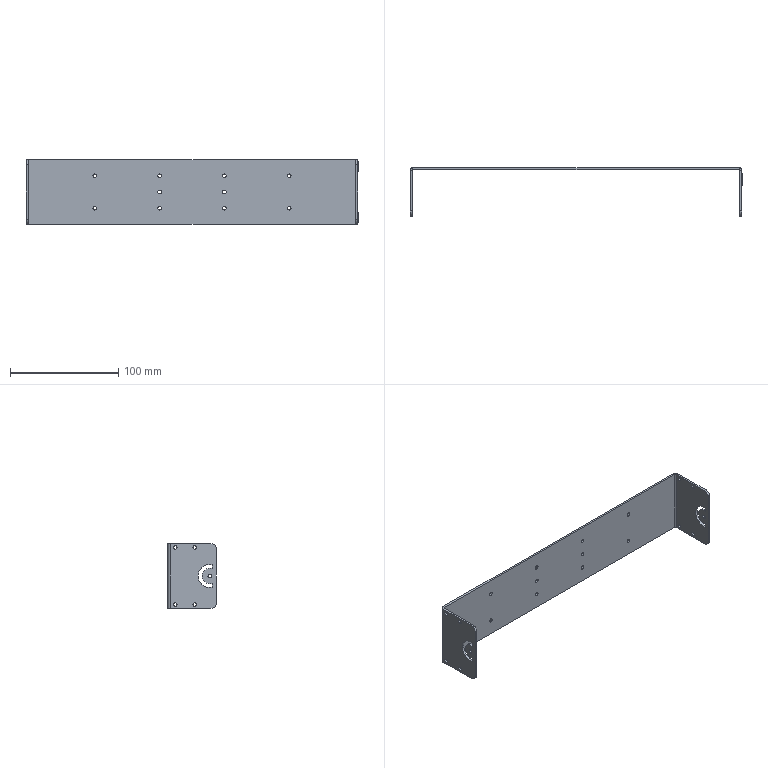Part | SolidWorks | features HoleWzd 2, ICE 2, EdgeFlange 1, Fillet 1, FlatPattern 1, SMBaseFlange 1, SheetMetal 1 | 1 solid | 74 faces | box 307 x 45 x 60 mm | volume 46139 mm3 | cylinder 52 | plane 22 | commonest cylinder face diameters 3.3 x36 3.5 x4 10 x4 1.473 x2 5.473 x2 14.5 x2